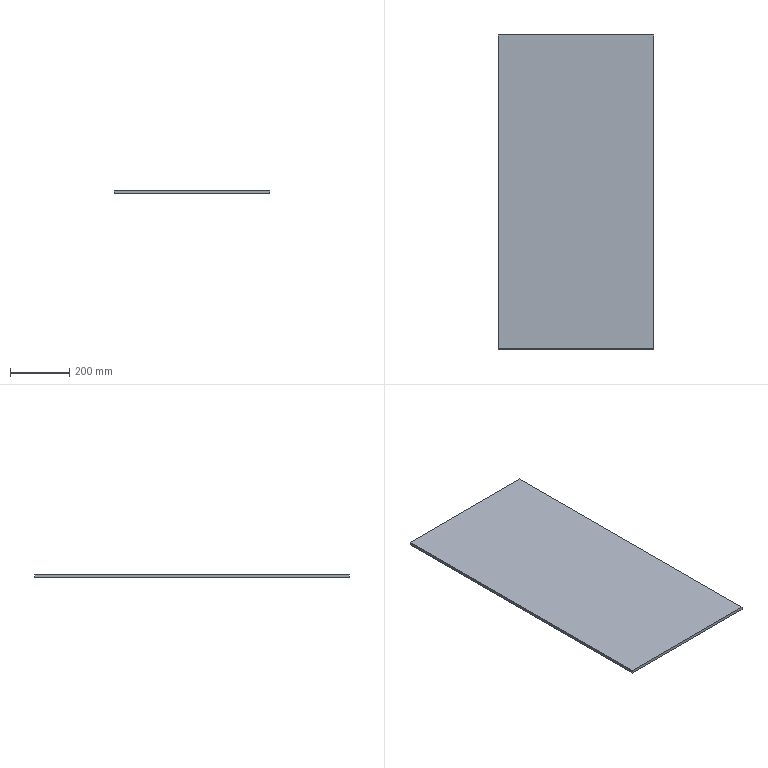Part | NX | features MOVE_FACE 3, BREP 1, DATUM_CSYS 1, DELETE FACE 1, SKETCH 1 | 1 solid | 6 faces | box 525 x 1060 x 10 mm | volume 5565000 mm3 | plane 6
STEP:
#1=CARTESIAN_POINT('',(-125.,120.,10.));
#2=VERTEX_POINT('',#1);
#3=CARTESIAN_POINT('',(-125.,-940.,10.));
#4=VERTEX_POINT('',#3);
#5=CARTESIAN_POINT('',(-125.,600.,10.));
#6=DIRECTION('',(0.,-1.,0.));
#7=VECTOR('',#6,1000.);
#8=LINE('',#5,#7);
#9=EDGE_CURVE('',#2,#4,#8,.T.);
#10=ORIENTED_EDGE('',*,*,#9,.T.);
#11=CARTESIAN_POINT('',(400.,-940.,10.));
#12=VERTEX_POINT('',#11);
#13=CARTESIAN_POINT('',(-400.,-940.,10.));
#14=DIRECTION('',(1.,0.,0.));
#15=VECTOR('',#14,1000.);
#16=LINE('',#13,#15);
#17=EDGE_CURVE('',#4,#12,#16,.T.);
#18=ORIENTED_EDGE('',*,*,#17,.T.);
#19=CARTESIAN_POINT('',(400.,120.,10.));
#20=VERTEX_POINT('',#19);
#21=CARTESIAN_POINT('',(400.,600.,10.));
#22=DIRECTION('',(0.,1.,0.));
#23=VECTOR('',#22,1000.);
#24=LINE('',#21,#23);
#25=EDGE_CURVE('',#12,#20,#24,.T.);
#26=ORIENTED_EDGE('',*,*,#25,.T.);
#27=CARTESIAN_POINT('',(-400.,120.,10.));
#28=DIRECTION('',(-1.,0.,0.));
#29=VECTOR('',#28,1000.);
#30=LINE('',#27,#29);
#31=EDGE_CURVE('',#20,#2,#30,.T.);
#32=ORIENTED_EDGE('',*,*,#31,.T.);
#33=EDGE_LOOP('',(#10,#18,#26,#32));
#34=FACE_BOUND('',#33,.T.);
#35=CARTESIAN_POINT('',(-400.,-600.,10.));
#36=DIRECTION('',(0.,0.,1.));
#37=DIRECTION('',(-1.,0.,0.));
#38=AXIS2_PLACEMENT_3D('',#35,#36,#37);
#39=PLANE('',#38);
#40=ADVANCED_FACE('',(#34),#39,.T.);
#41=CARTESIAN_POINT('',(-125.,120.,0.));
#42=VERTEX_POINT('',#41);
#43=CARTESIAN_POINT('',(-125.,-940.,0.));
#44=VERTEX_POINT('',#43);
#45=CARTESIAN_POINT('',(-125.,600.,0.));
#46=DIRECTION('',(0.,-1.,0.));
#47=VECTOR('',#46,1000.);
#48=LINE('',#45,#47);
#49=EDGE_CURVE('',#42,#44,#48,.T.);
#50=ORIENTED_EDGE('',*,*,#49,.F.);
#51=CARTESIAN_POINT('',(400.,120.,0.));
#52=VERTEX_POINT('',#51);
#53=CARTESIAN_POINT('',(-400.,120.,0.));
#54=DIRECTION('',(-1.,0.,0.));
#55=VECTOR('',#54,1000.);
#56=LINE('',#53,#55);
#57=EDGE_CURVE('',#52,#42,#56,.T.);
#58=ORIENTED_EDGE('',*,*,#57,.F.);
#59=CARTESIAN_POINT('',(400.,-940.,0.));
#60=VERTEX_POINT('',#59);
#61=CARTESIAN_POINT('',(400.,600.,0.));
#62=DIRECTION('',(0.,1.,0.));
#63=VECTOR('',#62,1000.);
#64=LINE('',#61,#63);
#65=EDGE_CURVE('',#60,#52,#64,.T.);
#66=ORIENTED_EDGE('',*,*,#65,.F.);
#67=CARTESIAN_POINT('',(-400.,-940.,0.));
#68=DIRECTION('',(1.,0.,0.));
#69=VECTOR('',#68,1000.);
#70=LINE('',#67,#69);
#71=EDGE_CURVE('',#44,#60,#70,.T.);
#72=ORIENTED_EDGE('',*,*,#71,.F.);
#73=EDGE_LOOP('',(#50,#58,#66,#72));
#74=FACE_BOUND('',#73,.T.);
#75=CARTESIAN_POINT('',(-400.,-600.,0.));
#76=DIRECTION('',(0.,0.,1.));
#77=DIRECTION('',(-1.,0.,0.));
#78=AXIS2_PLACEMENT_3D('',#75,#76,#77);
#79=PLANE('',#78);
#80=ADVANCED_FACE('',(#74),#79,.F.);
#81=ORIENTED_EDGE('',*,*,#49,.T.);
#82=CARTESIAN_POINT('',(-125.,-940.,10.));
#83=DIRECTION('',(0.,0.,-1.));
#84=VECTOR('',#83,1000.);
#85=LINE('',#82,#84);
#86=EDGE_CURVE('',#4,#44,#85,.T.);
#87=ORIENTED_EDGE('',*,*,#86,.F.);
#88=ORIENTED_EDGE('',*,*,#9,.F.);
#89=CARTESIAN_POINT('',(-125.,120.,10.));
#90=DIRECTION('',(0.,0.,-1.));
#91=VECTOR('',#90,1000.);
#92=LINE('',#89,#91);
#93=EDGE_CURVE('',#2,#42,#92,.T.);
#94=ORIENTED_EDGE('',*,*,#93,.T.);
#95=EDGE_LOOP('',(#81,#87,#88,#94));
#96=FACE_BOUND('',#95,.T.);
#97=CARTESIAN_POINT('',(-125.,600.,10.));
#98=DIRECTION('',(1.,0.,0.));
#99=DIRECTION('',(0.,0.,1.));
#100=AXIS2_PLACEMENT_3D('',#97,#98,#99);
#101=PLANE('',#100);
#102=ADVANCED_FACE('',(#96),#101,.F.);
#103=ORIENTED_EDGE('',*,*,#71,.T.);
#104=CARTESIAN_POINT('',(400.,-940.,10.));
#105=DIRECTION('',(0.,0.,-1.));
#106=VECTOR('',#105,1000.);
#107=LINE('',#104,#106);
#108=EDGE_CURVE('',#12,#60,#107,.T.);
#109=ORIENTED_EDGE('',*,*,#108,.F.);
#110=ORIENTED_EDGE('',*,*,#17,.F.);
#111=ORIENTED_EDGE('',*,*,#86,.T.);
#112=EDGE_LOOP('',(#103,#109,#110,#111));
#113=FACE_BOUND('',#112,.T.);
#114=CARTESIAN_POINT('',(-400.,-940.,10.));
#115=DIRECTION('',(0.,1.,0.));
#116=DIRECTION('',(0.,0.,-1.));
#117=AXIS2_PLACEMENT_3D('',#114,#115,#116);
#118=PLANE('',#117);
#119=ADVANCED_FACE('',(#113),#118,.F.);
#120=ORIENTED_EDGE('',*,*,#65,.T.);
#121=CARTESIAN_POINT('',(400.,120.,10.));
#122=DIRECTION('',(0.,0.,-1.));
#123=VECTOR('',#122,1000.);
#124=LINE('',#121,#123);
#125=EDGE_CURVE('',#20,#52,#124,.T.);
#126=ORIENTED_EDGE('',*,*,#125,.F.);
#127=ORIENTED_EDGE('',*,*,#25,.F.);
#128=ORIENTED_EDGE('',*,*,#108,.T.);
#129=EDGE_LOOP('',(#120,#126,#127,#128));
#130=FACE_BOUND('',#129,.T.);
#131=CARTESIAN_POINT('',(400.,600.,10.));
#132=DIRECTION('',(-1.,0.,0.));
#133=DIRECTION('',(0.,0.,-1.));
#134=AXIS2_PLACEMENT_3D('',#131,#132,#133);
#135=PLANE('',#134);
#136=ADVANCED_FACE('',(#130),#135,.F.);
#137=ORIENTED_EDGE('',*,*,#57,.T.);
#138=ORIENTED_EDGE('',*,*,#93,.F.);
#139=ORIENTED_EDGE('',*,*,#31,.F.);
#140=ORIENTED_EDGE('',*,*,#125,.T.);
#141=EDGE_LOOP('',(#137,#138,#139,#140));
#142=FACE_BOUND('',#141,.T.);
#143=CARTESIAN_POINT('',(-400.,120.,10.));
#144=DIRECTION('',(0.,-1.,0.));
#145=DIRECTION('',(0.,0.,1.));
#146=AXIS2_PLACEMENT_3D('',#143,#144,#145);
#147=PLANE('',#146);
#148=ADVANCED_FACE('',(#142),#147,.F.);
#149=CLOSED_SHELL('',(#40,#80,#102,#119,#136,#148));
#150=MANIFOLD_SOLID_BREP('',#149);
#151=(LENGTH_UNIT()NAMED_UNIT(*)SI_UNIT(.MILLI.,.METRE.));
#152=UNCERTAINTY_MEASURE_WITH_UNIT(LENGTH_MEASURE(0.00001),#151,'','');
#153=(NAMED_UNIT(*)PLANE_ANGLE_UNIT()SI_UNIT($,.RADIAN.));
#154=(NAMED_UNIT(*)SI_UNIT($,.STERADIAN.)SOLID_ANGLE_UNIT());
#155=(GEOMETRIC_REPRESENTATION_CONTEXT(3)GLOBAL_UNCERTAINTY_ASSIGNED_CONTEXT((#152))GLOBAL_UNIT_ASSIGNED_CONTEXT((#151,#153,#154))REPRESENTATION_CONTEXT('',''));
#156=ADVANCED_BREP_SHAPE_REPRESENTATION('',(#150),#155);